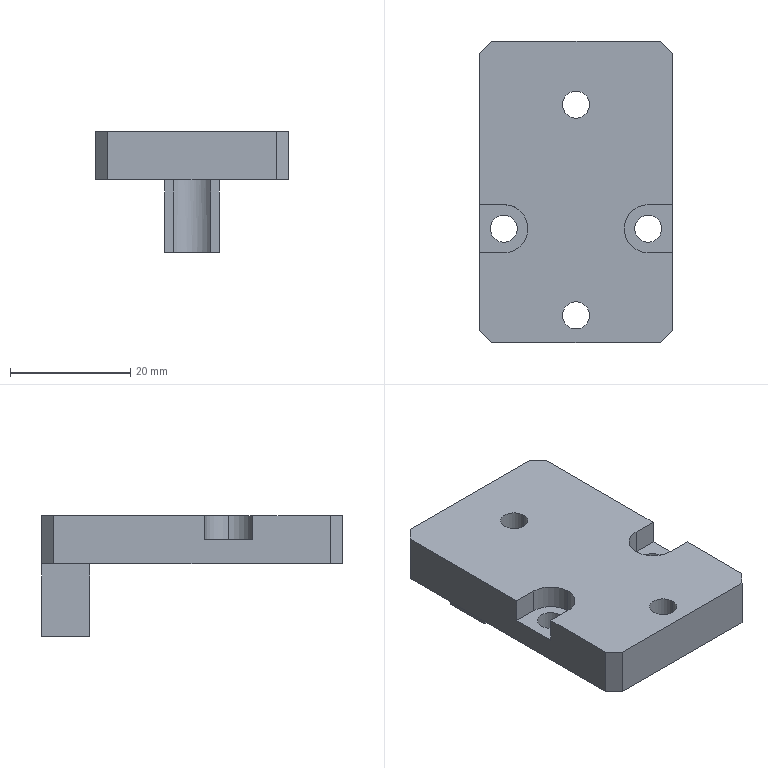Part | STEP file | 02-08 gripper limit block | 1 solid | 38 faces | box 32 x 50 x 20 mm | volume 12367 mm3 | plane 23 | cylinder 15 | commonest cylinder face diameters 4.5 x8 8 x7
STEP:
#1=CARTESIAN_POINT('',(4.,-20.5,16.6));
#2=VERTEX_POINT('',#1);
#3=CARTESIAN_POINT('',(-4.,-20.5,16.6));
#4=VERTEX_POINT('',#3);
#5=CARTESIAN_POINT('',(0.,-20.5,16.6));
#6=DIRECTION('',(0.,0.,-1.));
#7=DIRECTION('',(-1.,0.,0.));
#8=AXIS2_PLACEMENT_3D('',#5,#6,#7);
#9=CIRCLE('',#8,4.);
#10=EDGE_CURVE('',#2,#4,#9,.T.);
#11=ORIENTED_EDGE('',*,*,#10,.F.);
#12=CARTESIAN_POINT('',(4.,-20.5,12.));
#13=VERTEX_POINT('',#12);
#14=CARTESIAN_POINT('',(4.,-20.5,12.));
#15=DIRECTION('',(0.,0.,-1.));
#16=VECTOR('',#15,1000.);
#17=LINE('',#14,#16);
#18=EDGE_CURVE('',#2,#13,#17,.T.);
#19=ORIENTED_EDGE('',*,*,#18,.T.);
#20=CARTESIAN_POINT('',(-4.,-20.5,12.));
#21=VERTEX_POINT('',#20);
#22=CARTESIAN_POINT('',(0.,-20.5,12.));
#23=DIRECTION('',(0.,0.,-1.));
#24=DIRECTION('',(-1.,0.,0.));
#25=AXIS2_PLACEMENT_3D('',#22,#23,#24);
#26=CIRCLE('',#25,4.);
#27=EDGE_CURVE('',#13,#21,#26,.T.);
#28=ORIENTED_EDGE('',*,*,#27,.T.);
#29=CARTESIAN_POINT('',(-4.,-20.5,12.));
#30=DIRECTION('',(0.,0.,-1.));
#31=VECTOR('',#30,1000.);
#32=LINE('',#29,#31);
#33=EDGE_CURVE('',#4,#21,#32,.T.);
#34=ORIENTED_EDGE('',*,*,#33,.F.);
#35=EDGE_LOOP('',(#11,#19,#28,#34));
#36=FACE_OUTER_BOUND('',#35,.T.);
#37=CARTESIAN_POINT('',(0.,-20.5,12.));
#38=DIRECTION('',(0.,0.,-1.));
#39=DIRECTION('',(-1.,0.,0.));
#40=AXIS2_PLACEMENT_3D('',#37,#38,#39);
#41=CYLINDRICAL_SURFACE('',#40,4.);
#42=ADVANCED_FACE('',(#36),#41,.F.);
#43=CARTESIAN_POINT('',(2.25,-20.5,20.));
#44=VERTEX_POINT('',#43);
#45=CARTESIAN_POINT('',(-2.25,-20.5,20.));
#46=VERTEX_POINT('',#45);
#47=CARTESIAN_POINT('',(0.,-20.5,20.));
#48=DIRECTION('',(0.,0.,-1.));
#49=DIRECTION('',(-1.,0.,0.));
#50=AXIS2_PLACEMENT_3D('',#47,#48,#49);
#51=CIRCLE('',#50,2.25);
#52=EDGE_CURVE('',#44,#46,#51,.T.);
#53=ORIENTED_EDGE('',*,*,#52,.F.);
#54=CARTESIAN_POINT('',(2.25,-20.5,16.6));
#55=VERTEX_POINT('',#54);
#56=CARTESIAN_POINT('',(2.25,-20.5,12.));
#57=DIRECTION('',(0.,0.,-1.));
#58=VECTOR('',#57,1000.);
#59=LINE('',#56,#58);
#60=EDGE_CURVE('',#44,#55,#59,.T.);
#61=ORIENTED_EDGE('',*,*,#60,.T.);
#62=CARTESIAN_POINT('',(-2.25,-20.5,16.6));
#63=VERTEX_POINT('',#62);
#64=CARTESIAN_POINT('',(0.,-20.5,16.6));
#65=DIRECTION('',(0.,0.,-1.));
#66=DIRECTION('',(-1.,0.,0.));
#67=AXIS2_PLACEMENT_3D('',#64,#65,#66);
#68=CIRCLE('',#67,2.25);
#69=EDGE_CURVE('',#55,#63,#68,.T.);
#70=ORIENTED_EDGE('',*,*,#69,.T.);
#71=CARTESIAN_POINT('',(-2.25,-20.5,12.));
#72=DIRECTION('',(0.,0.,-1.));
#73=VECTOR('',#72,1000.);
#74=LINE('',#71,#73);
#75=EDGE_CURVE('',#46,#63,#74,.T.);
#76=ORIENTED_EDGE('',*,*,#75,.F.);
#77=EDGE_LOOP('',(#53,#61,#70,#76));
#78=FACE_OUTER_BOUND('',#77,.T.);
#79=CARTESIAN_POINT('',(0.,-20.5,12.));
#80=DIRECTION('',(0.,0.,-1.));
#81=DIRECTION('',(-1.,0.,0.));
#82=AXIS2_PLACEMENT_3D('',#79,#80,#81);
#83=CYLINDRICAL_SURFACE('',#82,2.25);
#84=ADVANCED_FACE('',(#78),#83,.F.);
#85=CARTESIAN_POINT('',(4.,14.5,16.6));
#86=VERTEX_POINT('',#85);
#87=CARTESIAN_POINT('',(-4.,14.5,16.6));
#88=VERTEX_POINT('',#87);
#89=CARTESIAN_POINT('',(0.,14.5,16.6));
#90=DIRECTION('',(0.,0.,-1.));
#91=DIRECTION('',(-1.,0.,0.));
#92=AXIS2_PLACEMENT_3D('',#89,#90,#91);
#93=CIRCLE('',#92,4.);
#94=EDGE_CURVE('',#86,#88,#93,.T.);
#95=ORIENTED_EDGE('',*,*,#94,.F.);
#96=CARTESIAN_POINT('',(4.,14.5,12.));
#97=VERTEX_POINT('',#96);
#98=CARTESIAN_POINT('',(4.,14.5,12.));
#99=DIRECTION('',(0.,0.,-1.));
#100=VECTOR('',#99,1000.);
#101=LINE('',#98,#100);
#102=EDGE_CURVE('',#86,#97,#101,.T.);
#103=ORIENTED_EDGE('',*,*,#102,.T.);
#104=CARTESIAN_POINT('',(-4.,14.5,12.));
#105=VERTEX_POINT('',#104);
#106=CARTESIAN_POINT('',(0.,14.5,12.));
#107=DIRECTION('',(0.,0.,-1.));
#108=DIRECTION('',(-1.,0.,0.));
#109=AXIS2_PLACEMENT_3D('',#106,#107,#108);
#110=CIRCLE('',#109,4.);
#111=EDGE_CURVE('',#97,#105,#110,.T.);
#112=ORIENTED_EDGE('',*,*,#111,.T.);
#113=CARTESIAN_POINT('',(-4.,14.5,12.));
#114=DIRECTION('',(0.,0.,-1.));
#115=VECTOR('',#114,1000.);
#116=LINE('',#113,#115);
#117=EDGE_CURVE('',#88,#105,#116,.T.);
#118=ORIENTED_EDGE('',*,*,#117,.F.);
#119=EDGE_LOOP('',(#95,#103,#112,#118));
#120=FACE_OUTER_BOUND('',#119,.T.);
#121=CARTESIAN_POINT('',(0.,14.5,12.));
#122=DIRECTION('',(0.,0.,-1.));
#123=DIRECTION('',(-1.,0.,0.));
#124=AXIS2_PLACEMENT_3D('',#121,#122,#123);
#125=CYLINDRICAL_SURFACE('',#124,4.);
#126=ADVANCED_FACE('',(#120),#125,.F.);
#127=CARTESIAN_POINT('',(2.25,14.5,20.));
#128=VERTEX_POINT('',#127);
#129=CARTESIAN_POINT('',(-2.25,14.5,20.));
#130=VERTEX_POINT('',#129);
#131=CARTESIAN_POINT('',(0.,14.5,20.));
#132=DIRECTION('',(0.,0.,-1.));
#133=DIRECTION('',(-1.,0.,0.));
#134=AXIS2_PLACEMENT_3D('',#131,#132,#133);
#135=CIRCLE('',#134,2.25);
#136=EDGE_CURVE('',#128,#130,#135,.T.);
#137=ORIENTED_EDGE('',*,*,#136,.F.);
#138=CARTESIAN_POINT('',(2.25,14.5,16.6));
#139=VERTEX_POINT('',#138);
#140=CARTESIAN_POINT('',(2.25,14.5,12.));
#141=DIRECTION('',(0.,0.,-1.));
#142=VECTOR('',#141,1000.);
#143=LINE('',#140,#142);
#144=EDGE_CURVE('',#128,#139,#143,.T.);
#145=ORIENTED_EDGE('',*,*,#144,.T.);
#146=CARTESIAN_POINT('',(-2.25,14.5,16.6));
#147=VERTEX_POINT('',#146);
#148=CARTESIAN_POINT('',(0.,14.5,16.6));
#149=DIRECTION('',(0.,0.,-1.));
#150=DIRECTION('',(-1.,0.,0.));
#151=AXIS2_PLACEMENT_3D('',#148,#149,#150);
#152=CIRCLE('',#151,2.25);
#153=EDGE_CURVE('',#139,#147,#152,.T.);
#154=ORIENTED_EDGE('',*,*,#153,.T.);
#155=CARTESIAN_POINT('',(-2.25,14.5,12.));
#156=DIRECTION('',(0.,0.,-1.));
#157=VECTOR('',#156,1000.);
#158=LINE('',#155,#157);
#159=EDGE_CURVE('',#130,#147,#158,.T.);
#160=ORIENTED_EDGE('',*,*,#159,.F.);
#161=EDGE_LOOP('',(#137,#145,#154,#160));
#162=FACE_OUTER_BOUND('',#161,.T.);
#163=CARTESIAN_POINT('',(0.,14.5,12.));
#164=DIRECTION('',(0.,0.,-1.));
#165=DIRECTION('',(-1.,0.,0.));
#166=AXIS2_PLACEMENT_3D('',#163,#164,#165);
#167=CYLINDRICAL_SURFACE('',#166,2.25);
#168=ADVANCED_FACE('',(#162),#167,.F.);
#169=CARTESIAN_POINT('',(-8.,-6.1,16.));
#170=VERTEX_POINT('',#169);
#171=CARTESIAN_POINT('',(-12.,-2.1,16.));
#172=VERTEX_POINT('',#171);
#173=CARTESIAN_POINT('',(-12.,-6.1,16.));
#174=DIRECTION('',(0.,0.,1.));
#175=DIRECTION('',(1.,0.,0.));
#176=AXIS2_PLACEMENT_3D('',#173,#174,#175);
#177=CIRCLE('',#176,4.);
#178=EDGE_CURVE('',#170,#172,#177,.T.);
#179=ORIENTED_EDGE('',*,*,#178,.F.);
#180=CARTESIAN_POINT('',(-8.,-6.1,20.));
#181=VERTEX_POINT('',#180);
#182=CARTESIAN_POINT('',(-8.,-6.1,16.));
#183=DIRECTION('',(0.,0.,1.));
#184=VECTOR('',#183,1000.);
#185=LINE('',#182,#184);
#186=EDGE_CURVE('',#170,#181,#185,.T.);
#187=ORIENTED_EDGE('',*,*,#186,.T.);
#188=CARTESIAN_POINT('',(-12.,-2.1,20.));
#189=VERTEX_POINT('',#188);
#190=CARTESIAN_POINT('',(-12.,-6.1,20.));
#191=DIRECTION('',(0.,0.,1.));
#192=DIRECTION('',(1.,0.,0.));
#193=AXIS2_PLACEMENT_3D('',#190,#191,#192);
#194=CIRCLE('',#193,4.);
#195=EDGE_CURVE('',#181,#189,#194,.T.);
#196=ORIENTED_EDGE('',*,*,#195,.T.);
#197=CARTESIAN_POINT('',(-12.,-2.1,16.));
#198=DIRECTION('',(0.,0.,1.));
#199=VECTOR('',#198,1000.);
#200=LINE('',#197,#199);
#201=EDGE_CURVE('',#172,#189,#200,.T.);
#202=ORIENTED_EDGE('',*,*,#201,.F.);
#203=EDGE_LOOP('',(#179,#187,#196,#202));
#204=FACE_OUTER_BOUND('',#203,.T.);
#205=CARTESIAN_POINT('',(-12.,-6.1,16.));
#206=DIRECTION('',(0.,0.,1.));
#207=DIRECTION('',(1.,0.,0.));
#208=AXIS2_PLACEMENT_3D('',#205,#206,#207);
#209=CYLINDRICAL_SURFACE('',#208,4.);
#210=ADVANCED_FACE('',(#204),#209,.F.);
#211=CARTESIAN_POINT('',(9.75,-6.1,12.));
#212=VERTEX_POINT('',#211);
#213=CARTESIAN_POINT('',(14.25,-6.1,12.));
#214=VERTEX_POINT('',#213);
#215=CARTESIAN_POINT('',(12.,-6.1,12.));
#216=DIRECTION('',(0.,0.,1.));
#217=DIRECTION('',(1.,0.,0.));
#218=AXIS2_PLACEMENT_3D('',#215,#216,#217);
#219=CIRCLE('',#218,2.25);
#220=EDGE_CURVE('',#212,#214,#219,.T.);
#221=ORIENTED_EDGE('',*,*,#220,.F.);
#222=CARTESIAN_POINT('',(9.75,-6.1,16.));
#223=VERTEX_POINT('',#222);
#224=CARTESIAN_POINT('',(9.75,-6.1,-10.));
#225=DIRECTION('',(0.,0.,1.));
#226=VECTOR('',#225,1000.);
#227=LINE('',#224,#226);
#228=EDGE_CURVE('',#212,#223,#227,.T.);
#229=ORIENTED_EDGE('',*,*,#228,.T.);
#230=CARTESIAN_POINT('',(14.25,-6.1,16.));
#231=VERTEX_POINT('',#230);
#232=CARTESIAN_POINT('',(12.,-6.1,16.));
#233=DIRECTION('',(0.,0.,-1.));
#234=DIRECTION('',(1.,0.,0.));
#235=AXIS2_PLACEMENT_3D('',#232,#233,#234);
#236=CIRCLE('',#235,2.25);
#237=EDGE_CURVE('',#231,#223,#236,.T.);
#238=ORIENTED_EDGE('',*,*,#237,.F.);
#239=CARTESIAN_POINT('',(14.25,-6.1,-10.));
#240=DIRECTION('',(0.,0.,1.));
#241=VECTOR('',#240,1000.);
#242=LINE('',#239,#241);
#243=EDGE_CURVE('',#214,#231,#242,.T.);
#244=ORIENTED_EDGE('',*,*,#243,.F.);
#245=EDGE_LOOP('',(#221,#229,#238,#244));
#246=FACE_OUTER_BOUND('',#245,.T.);
#247=CARTESIAN_POINT('',(12.,-6.1,-10.));
#248=DIRECTION('',(0.,0.,1.));
#249=DIRECTION('',(1.,0.,0.));
#250=AXIS2_PLACEMENT_3D('',#247,#248,#249);
#251=CYLINDRICAL_SURFACE('',#250,2.25);
#252=ADVANCED_FACE('',(#246),#251,.F.);
#253=CARTESIAN_POINT('',(-14.25,-6.1,12.));
#254=VERTEX_POINT('',#253);
#255=CARTESIAN_POINT('',(-9.75,-6.1,12.));
#256=VERTEX_POINT('',#255);
#257=CARTESIAN_POINT('',(-12.,-6.1,12.));
#258=DIRECTION('',(0.,0.,1.));
#259=DIRECTION('',(1.,0.,0.));
#260=AXIS2_PLACEMENT_3D('',#257,#258,#259);
#261=CIRCLE('',#260,2.25);
#262=EDGE_CURVE('',#254,#256,#261,.T.);
#263=ORIENTED_EDGE('',*,*,#262,.F.);
#264=CARTESIAN_POINT('',(-14.25,-6.1,16.));
#265=VERTEX_POINT('',#264);
#266=CARTESIAN_POINT('',(-14.25,-6.1,-10.));
#267=DIRECTION('',(0.,0.,1.));
#268=VECTOR('',#267,1000.);
#269=LINE('',#266,#268);
#270=EDGE_CURVE('',#254,#265,#269,.T.);
#271=ORIENTED_EDGE('',*,*,#270,.T.);
#272=CARTESIAN_POINT('',(-9.75,-6.1,16.));
#273=VERTEX_POINT('',#272);
#274=CARTESIAN_POINT('',(-12.,-6.1,16.));
#275=DIRECTION('',(0.,0.,-1.));
#276=DIRECTION('',(1.,0.,0.));
#277=AXIS2_PLACEMENT_3D('',#274,#275,#276);
#278=CIRCLE('',#277,2.25);
#279=EDGE_CURVE('',#273,#265,#278,.T.);
#280=ORIENTED_EDGE('',*,*,#279,.F.);
#281=CARTESIAN_POINT('',(-9.75,-6.1,-10.));
#282=DIRECTION('',(0.,0.,1.));
#283=VECTOR('',#282,1000.);
#284=LINE('',#281,#283);
#285=EDGE_CURVE('',#256,#273,#284,.T.);
#286=ORIENTED_EDGE('',*,*,#285,.F.);
#287=EDGE_LOOP('',(#263,#271,#280,#286));
#288=FACE_OUTER_BOUND('',#287,.T.);
#289=CARTESIAN_POINT('',(-12.,-6.1,-10.));
#290=DIRECTION('',(0.,0.,1.));
#291=DIRECTION('',(1.,0.,0.));
#292=AXIS2_PLACEMENT_3D('',#289,#290,#291);
#293=CYLINDRICAL_SURFACE('',#292,2.25);
#294=ADVANCED_FACE('',(#288),#293,.F.);
#295=CARTESIAN_POINT('',(-3.122,17.,0.));
#296=VERTEX_POINT('',#295);
#297=CARTESIAN_POINT('',(3.122,17.,0.));
#298=VERTEX_POINT('',#297);
#299=CARTESIAN_POINT('',(0.,14.5,0.));
#300=DIRECTION('',(0.,0.,-1.));
#301=DIRECTION('',(1.,0.,0.));
#302=AXIS2_PLACEMENT_3D('',#299,#300,#301);
#303=CIRCLE('',#302,4.);
#304=EDGE_CURVE('',#296,#298,#303,.T.);
#305=ORIENTED_EDGE('',*,*,#304,.F.);
#306=CARTESIAN_POINT('',(-4.5,17.,0.));
#307=VERTEX_POINT('',#306);
#308=CARTESIAN_POINT('',(34.,17.,0.));
#309=DIRECTION('',(-1.,0.,0.));
#310=VECTOR('',#309,1000.);
#311=LINE('',#308,#310);
#312=EDGE_CURVE('',#296,#307,#311,.T.);
#313=ORIENTED_EDGE('',*,*,#312,.T.);
#314=CARTESIAN_POINT('',(-4.5,25.,0.));
#315=VERTEX_POINT('',#314);
#316=CARTESIAN_POINT('',(-4.5,25.,0.));
#317=DIRECTION('',(0.,1.,0.));
#318=VECTOR('',#317,1000.);
#319=LINE('',#316,#318);
#320=EDGE_CURVE('',#307,#315,#319,.T.);
#321=ORIENTED_EDGE('',*,*,#320,.T.);
#322=CARTESIAN_POINT('',(4.5,25.,0.));
#323=VERTEX_POINT('',#322);
#324=CARTESIAN_POINT('',(-16.,25.,0.));
#325=DIRECTION('',(-1.,0.,0.));
#326=VECTOR('',#325,1000.);
#327=LINE('',#324,#326);
#328=EDGE_CURVE('',#323,#315,#327,.T.);
#329=ORIENTED_EDGE('',*,*,#328,.F.);
#330=CARTESIAN_POINT('',(4.5,17.,0.));
#331=VERTEX_POINT('',#330);
#332=CARTESIAN_POINT('',(4.5,25.,0.));
#333=DIRECTION('',(0.,-1.,0.));
#334=VECTOR('',#333,1000.);
#335=LINE('',#332,#334);
#336=EDGE_CURVE('',#323,#331,#335,.T.);
#337=ORIENTED_EDGE('',*,*,#336,.T.);
#338=CARTESIAN_POINT('',(34.,17.,0.));
#339=DIRECTION('',(-1.,0.,0.));
#340=VECTOR('',#339,1000.);
#341=LINE('',#338,#340);
#342=EDGE_CURVE('',#331,#298,#341,.T.);
#343=ORIENTED_EDGE('',*,*,#342,.T.);
#344=EDGE_LOOP('',(#305,#313,#321,#329,#337,#343));
#345=FACE_OUTER_BOUND('',#344,.T.);
#346=CARTESIAN_POINT('',(16.,-25.,0.));
#347=DIRECTION('',(0.,0.,1.));
#348=DIRECTION('',(1.,0.,0.));
#349=AXIS2_PLACEMENT_3D('',#346,#347,#348);
#350=PLANE('',#349);
#351=ADVANCED_FACE('',(#345),#350,.F.);
#352=CARTESIAN_POINT('',(-3.122,17.,12.));
#353=VERTEX_POINT('',#352);
#354=CARTESIAN_POINT('',(-3.122,17.,-2.4));
#355=DIRECTION('',(0.,0.,-1.));
#356=VECTOR('',#355,1000.);
#357=LINE('',#354,#356);
#358=EDGE_CURVE('',#353,#296,#357,.T.);
#359=ORIENTED_EDGE('',*,*,#358,.F.);
#360=CARTESIAN_POINT('',(-4.5,17.,12.));
#361=VERTEX_POINT('',#360);
#362=CARTESIAN_POINT('',(34.,17.,12.));
#363=DIRECTION('',(-1.,0.,0.));
#364=VECTOR('',#363,1000.);
#365=LINE('',#362,#364);
#366=EDGE_CURVE('',#353,#361,#365,.T.);
#367=ORIENTED_EDGE('',*,*,#366,.T.);
#368=CARTESIAN_POINT('',(-4.5,17.,0.));
#369=DIRECTION('',(0.,0.,1.));
#370=VECTOR('',#369,1000.);
#371=LINE('',#368,#370);
#372=EDGE_CURVE('',#307,#361,#371,.T.);
#373=ORIENTED_EDGE('',*,*,#372,.F.);
#374=ORIENTED_EDGE('',*,*,#312,.F.);
#375=EDGE_LOOP('',(#359,#367,#373,#374));
#376=FACE_OUTER_BOUND('',#375,.T.);
#377=CARTESIAN_POINT('',(34.,17.,0.));
#378=DIRECTION('',(0.,1.,0.));
#379=DIRECTION('',(-1.,0.,0.));
#380=AXIS2_PLACEMENT_3D('',#377,#378,#379);
#381=PLANE('',#380);
#382=ADVANCED_FACE('',(#376),#381,.F.);
#383=CARTESIAN_POINT('',(3.122,17.,12.));
#384=VERTEX_POINT('',#383);
#385=CARTESIAN_POINT('',(3.122,17.,-2.4));
#386=DIRECTION('',(0.,0.,1.));
#387=VECTOR('',#386,1000.);
#388=LINE('',#385,#387);
#389=EDGE_CURVE('',#298,#384,#388,.T.);
#390=ORIENTED_EDGE('',*,*,#389,.F.);
#391=ORIENTED_EDGE('',*,*,#342,.F.);
#392=CARTESIAN_POINT('',(4.5,17.,12.));
#393=VERTEX_POINT('',#392);
#394=CARTESIAN_POINT('',(4.5,17.,0.));
#395=DIRECTION('',(0.,0.,-1.));
#396=VECTOR('',#395,1000.);
#397=LINE('',#394,#396);
#398=EDGE_CURVE('',#393,#331,#397,.T.);
#399=ORIENTED_EDGE('',*,*,#398,.F.);
#400=CARTESIAN_POINT('',(34.,17.,12.));
#401=DIRECTION('',(-1.,0.,0.));
#402=VECTOR('',#401,1000.);
#403=LINE('',#400,#402);
#404=EDGE_CURVE('',#393,#384,#403,.T.);
#405=ORIENTED_EDGE('',*,*,#404,.T.);
#406=EDGE_LOOP('',(#390,#391,#399,#405));
#407=FACE_OUTER_BOUND('',#406,.T.);
#408=CARTESIAN_POINT('',(34.,17.,0.));
#409=DIRECTION('',(0.,1.,0.));
#410=DIRECTION('',(-1.,0.,0.));
#411=AXIS2_PLACEMENT_3D('',#408,#409,#410);
#412=PLANE('',#411);
#413=ADVANCED_FACE('',(#407),#412,.F.);
#414=CARTESIAN_POINT('',(0.,-20.5,12.));
#415=DIRECTION('',(0.,0.,-1.));
#416=DIRECTION('',(-1.,0.,0.));
#417=AXIS2_PLACEMENT_3D('',#414,#415,#416);
#418=CIRCLE('',#417,4.);
#419=EDGE_CURVE('',#21,#13,#418,.T.);
#420=ORIENTED_EDGE('',*,*,#419,.F.);
#421=ORIENTED_EDGE('',*,*,#27,.F.);
#422=EDGE_LOOP('',(#420,#421));
#423=FACE_BOUND('',#422,.T.);
#424=CARTESIAN_POINT('',(12.,-6.1,12.));
#425=DIRECTION('',(0.,0.,1.));
#426=DIRECTION('',(1.,0.,0.));
#427=AXIS2_PLACEMENT_3D('',#424,#425,#426);
#428=CIRCLE('',#427,2.25);
#429=EDGE_CURVE('',#214,#212,#428,.T.);
#430=ORIENTED_EDGE('',*,*,#429,.T.);
#431=ORIENTED_EDGE('',*,*,#220,.T.);
#432=EDGE_LOOP('',(#430,#431));
#433=FACE_BOUND('',#432,.T.);
#434=CARTESIAN_POINT('',(-12.,-6.1,12.));
#435=DIRECTION('',(0.,0.,1.));
#436=DIRECTION('',(1.,0.,0.));
#437=AXIS2_PLACEMENT_3D('',#434,#435,#436);
#438=CIRCLE('',#437,2.25);
#439=EDGE_CURVE('',#256,#254,#438,.T.);
#440=ORIENTED_EDGE('',*,*,#439,.T.);
#441=ORIENTED_EDGE('',*,*,#262,.T.);
#442=EDGE_LOOP('',(#440,#441));
#443=FACE_BOUND('',#442,.T.);
#444=CARTESIAN_POINT('',(0.,14.5,12.));
#445=DIRECTION('',(0.,0.,-1.));
#446=DIRECTION('',(-1.,0.,0.));
#447=AXIS2_PLACEMENT_3D('',#444,#445,#446);
#448=CIRCLE('',#447,4.);
#449=EDGE_CURVE('',#384,#97,#448,.T.);
#450=ORIENTED_EDGE('',*,*,#449,.F.);
#451=ORIENTED_EDGE('',*,*,#404,.F.);
#452=CARTESIAN_POINT('',(4.5,25.,12.));
#453=VERTEX_POINT('',#452);
#454=CARTESIAN_POINT('',(4.5,25.,12.));
#455=DIRECTION('',(0.,1.,0.));
#456=VECTOR('',#455,1000.);
#457=LINE('',#454,#456);
#458=EDGE_CURVE('',#393,#453,#457,.T.);
#459=ORIENTED_EDGE('',*,*,#458,.T.);
#460=CARTESIAN_POINT('',(14.,25.,12.));
#461=VERTEX_POINT('',#460);
#462=CARTESIAN_POINT('',(16.,25.,12.));
#463=DIRECTION('',(1.,0.,0.));
#464=VECTOR('',#463,1000.);
#465=LINE('',#462,#464);
#466=EDGE_CURVE('',#453,#461,#465,.T.);
#467=ORIENTED_EDGE('',*,*,#466,.T.);
#468=CARTESIAN_POINT('',(16.,23.,12.));
#469=VERTEX_POINT('',#468);
#470=CARTESIAN_POINT('',(14.,25.,12.));
#471=DIRECTION('',(0.7071,-0.7071,0.));
#472=VECTOR('',#471,1000.);
#473=LINE('',#470,#472);
#474=EDGE_CURVE('',#461,#469,#473,.T.);
#475=ORIENTED_EDGE('',*,*,#474,.T.);
#476=CARTESIAN_POINT('',(16.,-23.,12.));
#477=VERTEX_POINT('',#476);
#478=CARTESIAN_POINT('',(16.,25.,12.));
#479=DIRECTION('',(0.,1.,0.));
#480=VECTOR('',#479,1000.);
#481=LINE('',#478,#480);
#482=EDGE_CURVE('',#477,#469,#481,.T.);
#483=ORIENTED_EDGE('',*,*,#482,.F.);
#484=CARTESIAN_POINT('',(14.,-25.,12.));
#485=VERTEX_POINT('',#484);
#486=CARTESIAN_POINT('',(16.,-23.,12.));
#487=DIRECTION('',(-0.7071,-0.7071,0.));
#488=VECTOR('',#487,1000.);
#489=LINE('',#486,#488);
#490=EDGE_CURVE('',#477,#485,#489,.T.);
#491=ORIENTED_EDGE('',*,*,#490,.T.);
#492=CARTESIAN_POINT('',(-14.,-25.,12.));
#493=VERTEX_POINT('',#492);
#494=CARTESIAN_POINT('',(34.,-25.,12.));
#495=DIRECTION('',(-1.,0.,0.));
#496=VECTOR('',#495,1000.);
#497=LINE('',#494,#496);
#498=EDGE_CURVE('',#485,#493,#497,.T.);
#499=ORIENTED_EDGE('',*,*,#498,.T.);
#500=CARTESIAN_POINT('',(-16.,-23.,12.));
#501=VERTEX_POINT('',#500);
#502=CARTESIAN_POINT('',(-14.,-25.,12.));
#503=DIRECTION('',(-0.7071,0.7071,0.));
#504=VECTOR('',#503,1000.);
#505=LINE('',#502,#504);
#506=EDGE_CURVE('',#493,#501,#505,.T.);
#507=ORIENTED_EDGE('',*,*,#506,.T.);
#508=CARTESIAN_POINT('',(-16.,23.,12.));
#509=VERTEX_POINT('',#508);
#510=CARTESIAN_POINT('',(-16.,-25.,12.));
#511=DIRECTION('',(0.,1.,0.));
#512=VECTOR('',#511,1000.);
#513=LINE('',#510,#512);
#514=EDGE_CURVE('',#501,#509,#513,.T.);
#515=ORIENTED_EDGE('',*,*,#514,.T.);
#516=CARTESIAN_POINT('',(-14.,25.,12.));
#517=VERTEX_POINT('',#516);
#518=CARTESIAN_POINT('',(-16.,23.,12.));
#519=DIRECTION('',(0.7071,0.7071,0.));
#520=VECTOR('',#519,1000.);
#521=LINE('',#518,#520);
#522=EDGE_CURVE('',#509,#517,#521,.T.);
#523=ORIENTED_EDGE('',*,*,#522,.T.);
#524=CARTESIAN_POINT('',(-4.5,25.,12.));
#525=VERTEX_POINT('',#524);
#526=CARTESIAN_POINT('',(16.,25.,12.));
#527=DIRECTION('',(1.,0.,0.));
#528=VECTOR('',#527,1000.);
#529=LINE('',#526,#528);
#530=EDGE_CURVE('',#517,#525,#529,.T.);
#531=ORIENTED_EDGE('',*,*,#530,.T.);
#532=CARTESIAN_POINT('',(-4.5,25.,12.));
#533=DIRECTION('',(0.,-1.,0.));
#534=VECTOR('',#533,1000.);
#535=LINE('',#532,#534);
#536=EDGE_CURVE('',#525,#361,#535,.T.);
#537=ORIENTED_EDGE('',*,*,#536,.T.);
#538=ORIENTED_EDGE('',*,*,#366,.F.);
#539=CARTESIAN_POINT('',(0.,14.5,12.));
#540=DIRECTION('',(0.,0.,-1.));
#541=DIRECTION('',(-1.,0.,0.));
#542=AXIS2_PLACEMENT_3D('',#539,#540,#541);
#543=CIRCLE('',#542,4.);
#544=EDGE_CURVE('',#105,#353,#543,.T.);
#545=ORIENTED_EDGE('',*,*,#544,.F.);
#546=ORIENTED_EDGE('',*,*,#111,.F.);
#547=EDGE_LOOP('',(#450,#451,#459,#467,#475,#483,#491,#499,#507,#515,#523,#531,#537,#538,#545,#546));
#548=FACE_OUTER_BOUND('',#547,.T.);
#549=CARTESIAN_POINT('',(34.,-25.,12.));
#550=DIRECTION('',(0.,0.,1.));
#551=DIRECTION('',(1.,0.,0.));
#552=AXIS2_PLACEMENT_3D('',#549,#550,#551);
#553=PLANE('',#552);
#554=ADVANCED_FACE('',(#423,#433,#443,#548),#553,.F.);
#555=ORIENTED_EDGE('',*,*,#458,.F.);
#556=ORIENTED_EDGE('',*,*,#398,.T.);
#557=ORIENTED_EDGE('',*,*,#336,.F.);
#558=CARTESIAN_POINT('',(4.5,25.,0.));
#559=DIRECTION('',(0.,0.,1.));
#560=VECTOR('',#559,1000.);
#561=LINE('',#558,#560);
#562=EDGE_CURVE('',#323,#453,#561,.T.);
#563=ORIENTED_EDGE('',*,*,#562,.T.);
#564=EDGE_LOOP('',(#555,#556,#557,#563));
#565=FACE_OUTER_BOUND('',#564,.T.);
#566=CARTESIAN_POINT('',(4.5,25.,0.));
#567=DIRECTION('',(-1.,0.,0.));
#568=DIRECTION('',(0.,-1.,0.));
#569=AXIS2_PLACEMENT_3D('',#566,#567,#568);
#570=PLANE('',#569);
#571=ADVANCED_FACE('',(#565),#570,.F.);
#572=ORIENTED_EDGE('',*,*,#536,.F.);
#573=CARTESIAN_POINT('',(-4.5,25.,0.));
#574=DIRECTION('',(0.,0.,1.));
#575=VECTOR('',#574,1000.);
#576=LINE('',#573,#575);
#577=EDGE_CURVE('',#315,#525,#576,.T.);
#578=ORIENTED_EDGE('',*,*,#577,.F.);
#579=ORIENTED_EDGE('',*,*,#320,.F.);
#580=ORIENTED_EDGE('',*,*,#372,.T.);
#581=EDGE_LOOP('',(#572,#578,#579,#580));
#582=FACE_OUTER_BOUND('',#581,.T.);
#583=CARTESIAN_POINT('',(-4.5,25.,0.));
#584=DIRECTION('',(1.,0.,0.));
#585=DIRECTION('',(0.,1.,0.));
#586=AXIS2_PLACEMENT_3D('',#583,#584,#585);
#587=PLANE('',#586);
#588=ADVANCED_FACE('',(#582),#587,.F.);
#589=ORIENTED_EDGE('',*,*,#270,.F.);
#590=ORIENTED_EDGE('',*,*,#439,.F.);
#591=ORIENTED_EDGE('',*,*,#285,.T.);
#592=CARTESIAN_POINT('',(-12.,-6.1,16.));
#593=DIRECTION('',(0.,0.,-1.));
#594=DIRECTION('',(1.,0.,0.));
#595=AXIS2_PLACEMENT_3D('',#592,#593,#594);
#596=CIRCLE('',#595,2.25);
#597=EDGE_CURVE('',#265,#273,#596,.T.);
#598=ORIENTED_EDGE('',*,*,#597,.F.);
#599=EDGE_LOOP('',(#589,#590,#591,#598));
#600=FACE_OUTER_BOUND('',#599,.T.);
#601=CARTESIAN_POINT('',(-12.,-6.1,-10.));
#602=DIRECTION('',(0.,0.,1.));
#603=DIRECTION('',(1.,0.,0.));
#604=AXIS2_PLACEMENT_3D('',#601,#602,#603);
#605=CYLINDRICAL_SURFACE('',#604,2.25);
#606=ADVANCED_FACE('',(#600),#605,.F.);
#607=ORIENTED_EDGE('',*,*,#228,.F.);
#608=ORIENTED_EDGE('',*,*,#429,.F.);
#609=ORIENTED_EDGE('',*,*,#243,.T.);
#610=CARTESIAN_POINT('',(12.,-6.1,16.));
#611=DIRECTION('',(0.,0.,-1.));
#612=DIRECTION('',(1.,0.,0.));
#613=AXIS2_PLACEMENT_3D('',#610,#611,#612);
#614=CIRCLE('',#613,2.25);
#615=EDGE_CURVE('',#223,#231,#614,.T.);
#616=ORIENTED_EDGE('',*,*,#615,.F.);
#617=EDGE_LOOP('',(#607,#608,#609,#616));
#618=FACE_OUTER_BOUND('',#617,.T.);
#619=CARTESIAN_POINT('',(12.,-6.1,-10.));
#620=DIRECTION('',(0.,0.,1.));
#621=DIRECTION('',(1.,0.,0.));
#622=AXIS2_PLACEMENT_3D('',#619,#620,#621);
#623=CYLINDRICAL_SURFACE('',#622,2.25);
#624=ADVANCED_FACE('',(#618),#623,.F.);
#625=CARTESIAN_POINT('',(16.,-23.,20.));
#626=VERTEX_POINT('',#625);
#627=CARTESIAN_POINT('',(16.,-10.1,20.));
#628=VERTEX_POINT('',#627);
#629=CARTESIAN_POINT('',(16.,25.,20.));
#630=DIRECTION('',(0.,1.,0.));
#631=VECTOR('',#630,1000.);
#632=LINE('',#629,#631);
#633=EDGE_CURVE('',#626,#628,#632,.T.);
#634=ORIENTED_EDGE('',*,*,#633,.F.);
#635=CARTESIAN_POINT('',(16.,-23.,20.));
#636=DIRECTION('',(0.,0.,-1.));
#637=VECTOR('',#636,1000.);
#638=LINE('',#635,#637);
#639=EDGE_CURVE('',#626,#477,#638,.T.);
#640=ORIENTED_EDGE('',*,*,#639,.T.);
#641=ORIENTED_EDGE('',*,*,#482,.T.);
#642=CARTESIAN_POINT('',(16.,23.,20.));
#643=VERTEX_POINT('',#642);
#644=CARTESIAN_POINT('',(16.,23.,20.));
#645=DIRECTION('',(0.,0.,1.));
#646=VECTOR('',#645,1000.);
#647=LINE('',#644,#646);
#648=EDGE_CURVE('',#469,#643,#647,.T.);
#649=ORIENTED_EDGE('',*,*,#648,.T.);
#650=CARTESIAN_POINT('',(16.,-2.1,20.));
#651=VERTEX_POINT('',#650);
#652=CARTESIAN_POINT('',(16.,25.,20.));
#653=DIRECTION('',(0.,1.,0.));
#654=VECTOR('',#653,1000.);
#655=LINE('',#652,#654);
#656=EDGE_CURVE('',#651,#643,#655,.T.);
#657=ORIENTED_EDGE('',*,*,#656,.F.);
#658=CARTESIAN_POINT('',(16.,-2.1,16.));
#659=VERTEX_POINT('',#658);
#660=CARTESIAN_POINT('',(16.,-2.1,20.));
#661=DIRECTION('',(0.,0.,-1.));
#662=VECTOR('',#661,1000.);
#663=LINE('',#660,#662);
#664=EDGE_CURVE('',#651,#659,#663,.T.);
#665=ORIENTED_EDGE('',*,*,#664,.T.);
#666=CARTESIAN_POINT('',(16.,-10.1,16.));
#667=VERTEX_POINT('',#666);
#668=CARTESIAN_POINT('',(16.,25.,16.));
#669=DIRECTION('',(0.,1.,0.));
#670=VECTOR('',#669,1000.);
#671=LINE('',#668,#670);
#672=EDGE_CURVE('',#667,#659,#671,.T.);
#673=ORIENTED_EDGE('',*,*,#672,.F.);
#674=CARTESIAN_POINT('',(16.,-10.1,20.));
#675=DIRECTION('',(0.,0.,1.));
#676=VECTOR('',#675,1000.);
#677=LINE('',#674,#676);
#678=EDGE_CURVE('',#667,#628,#677,.T.);
#679=ORIENTED_EDGE('',*,*,#678,.T.);
#680=EDGE_LOOP('',(#634,#640,#641,#649,#657,#665,#673,#679));
#681=FACE_OUTER_BOUND('',#680,.T.);
#682=CARTESIAN_POINT('',(16.,25.,20.));
#683=DIRECTION('',(-1.,0.,0.));
#684=DIRECTION('',(0.,-1.,0.));
#685=AXIS2_PLACEMENT_3D('',#682,#683,#684);
#686=PLANE('',#685);
#687=ADVANCED_FACE('',(#681),#686,.F.);
#688=CARTESIAN_POINT('',(14.,25.,20.));
#689=VERTEX_POINT('',#688);
#690=CARTESIAN_POINT('',(-14.,25.,20.));
#691=VERTEX_POINT('',#690);
#692=CARTESIAN_POINT('',(-16.,25.,20.));
#693=DIRECTION('',(-1.,0.,0.));
#694=VECTOR('',#693,1000.);
#695=LINE('',#692,#694);
#696=EDGE_CURVE('',#689,#691,#695,.T.);
#697=ORIENTED_EDGE('',*,*,#696,.F.);
#698=CARTESIAN_POINT('',(14.,25.,20.));
#699=DIRECTION('',(0.,0.,-1.));
#700=VECTOR('',#699,1000.);
#701=LINE('',#698,#700);
#702=EDGE_CURVE('',#689,#461,#701,.T.);
#703=ORIENTED_EDGE('',*,*,#702,.T.);
#704=ORIENTED_EDGE('',*,*,#466,.F.);
#705=ORIENTED_EDGE('',*,*,#562,.F.);
#706=ORIENTED_EDGE('',*,*,#328,.T.);
#707=ORIENTED_EDGE('',*,*,#577,.T.);
#708=ORIENTED_EDGE('',*,*,#530,.F.);
#709=CARTESIAN_POINT('',(-14.,25.,20.));
#710=DIRECTION('',(0.,0.,1.));
#711=VECTOR('',#710,1000.);
#712=LINE('',#709,#711);
#713=EDGE_CURVE('',#517,#691,#712,.T.);
#714=ORIENTED_EDGE('',*,*,#713,.T.);
#715=EDGE_LOOP('',(#697,#703,#704,#705,#706,#707,#708,#714));
#716=FACE_OUTER_BOUND('',#715,.T.);
#717=CARTESIAN_POINT('',(-16.,25.,20.));
#718=DIRECTION('',(0.,-1.,0.));
#719=DIRECTION('',(0.,0.,-1.));
#720=AXIS2_PLACEMENT_3D('',#717,#718,#719);
#721=PLANE('',#720);
#722=ADVANCED_FACE('',(#716),#721,.F.);
#723=ORIENTED_EDGE('',*,*,#514,.F.);
#724=CARTESIAN_POINT('',(-16.,-23.,20.));
#725=VERTEX_POINT('',#724);
#726=CARTESIAN_POINT('',(-16.,-23.,20.));
#727=DIRECTION('',(0.,0.,1.));
#728=VECTOR('',#727,1000.);
#729=LINE('',#726,#728);
#730=EDGE_CURVE('',#501,#725,#729,.T.);
#731=ORIENTED_EDGE('',*,*,#730,.T.);
#732=CARTESIAN_POINT('',(-16.,-10.1,20.));
#733=VERTEX_POINT('',#732);
#734=CARTESIAN_POINT('',(-16.,25.,20.));
#735=DIRECTION('',(0.,-1.,0.));
#736=VECTOR('',#735,1000.);
#737=LINE('',#734,#736);
#738=EDGE_CURVE('',#733,#725,#737,.T.);
#739=ORIENTED_EDGE('',*,*,#738,.F.);
#740=CARTESIAN_POINT('',(-16.,-10.1,16.));
#741=VERTEX_POINT('',#740);
#742=CARTESIAN_POINT('',(-16.,-10.1,20.));
#743=DIRECTION('',(0.,0.,-1.));
#744=VECTOR('',#743,1000.);
#745=LINE('',#742,#744);
#746=EDGE_CURVE('',#733,#741,#745,.T.);
#747=ORIENTED_EDGE('',*,*,#746,.T.);
#748=CARTESIAN_POINT('',(-16.,-2.1,16.));
#749=VERTEX_POINT('',#748);
#750=CARTESIAN_POINT('',(-16.,25.,16.));
#751=DIRECTION('',(0.,-1.,0.));
#752=VECTOR('',#751,1000.);
#753=LINE('',#750,#752);
#754=EDGE_CURVE('',#749,#741,#753,.T.);
#755=ORIENTED_EDGE('',*,*,#754,.F.);
#756=CARTESIAN_POINT('',(-16.,-2.1,20.));
#757=VERTEX_POINT('',#756);
#758=CARTESIAN_POINT('',(-16.,-2.1,20.));
#759=DIRECTION('',(0.,0.,1.));
#760=VECTOR('',#759,1000.);
#761=LINE('',#758,#760);
#762=EDGE_CURVE('',#749,#757,#761,.T.);
#763=ORIENTED_EDGE('',*,*,#762,.T.);
#764=CARTESIAN_POINT('',(-16.,23.,20.));
#765=VERTEX_POINT('',#764);
#766=CARTESIAN_POINT('',(-16.,25.,20.));
#767=DIRECTION('',(0.,-1.,0.));
#768=VECTOR('',#767,1000.);
#769=LINE('',#766,#768);
#770=EDGE_CURVE('',#765,#757,#769,.T.);
#771=ORIENTED_EDGE('',*,*,#770,.F.);
#772=CARTESIAN_POINT('',(-16.,23.,20.));
#773=DIRECTION('',(0.,0.,-1.));
#774=VECTOR('',#773,1000.);
#775=LINE('',#772,#774);
#776=EDGE_CURVE('',#765,#509,#775,.T.);
#777=ORIENTED_EDGE('',*,*,#776,.T.);
#778=EDGE_LOOP('',(#723,#731,#739,#747,#755,#763,#771,#777));
#779=FACE_OUTER_BOUND('',#778,.T.);
#780=CARTESIAN_POINT('',(-16.,25.,20.));
#781=DIRECTION('',(1.,0.,0.));
#782=DIRECTION('',(0.,1.,0.));
#783=AXIS2_PLACEMENT_3D('',#780,#781,#782);
#784=PLANE('',#783);
#785=ADVANCED_FACE('',(#779),#784,.F.);
#786=CARTESIAN_POINT('',(-14.,-25.,20.));
#787=VERTEX_POINT('',#786);
#788=CARTESIAN_POINT('',(14.,-25.,20.));
#789=VERTEX_POINT('',#788);
#790=CARTESIAN_POINT('',(-16.,-25.,20.));
#791=DIRECTION('',(1.,0.,0.));
#792=VECTOR('',#791,1000.);
#793=LINE('',#790,#792);
#794=EDGE_CURVE('',#787,#789,#793,.T.);
#795=ORIENTED_EDGE('',*,*,#794,.F.);
#796=CARTESIAN_POINT('',(-14.,-25.,20.));
#797=DIRECTION('',(0.,0.,-1.));
#798=VECTOR('',#797,1000.);
#799=LINE('',#796,#798);
#800=EDGE_CURVE('',#787,#493,#799,.T.);
#801=ORIENTED_EDGE('',*,*,#800,.T.);
#802=ORIENTED_EDGE('',*,*,#498,.F.);
#803=CARTESIAN_POINT('',(14.,-25.,20.));
#804=DIRECTION('',(0.,0.,1.));
#805=VECTOR('',#804,1000.);
#806=LINE('',#803,#805);
#807=EDGE_CURVE('',#485,#789,#806,.T.);
#808=ORIENTED_EDGE('',*,*,#807,.T.);
#809=EDGE_LOOP('',(#795,#801,#802,#808));
#810=FACE_OUTER_BOUND('',#809,.T.);
#811=CARTESIAN_POINT('',(-16.,-25.,20.));
#812=DIRECTION('',(0.,1.,0.));
#813=DIRECTION('',(0.,0.,1.));
#814=AXIS2_PLACEMENT_3D('',#811,#812,#813);
#815=PLANE('',#814);
#816=ADVANCED_FACE('',(#810),#815,.F.);
#817=CARTESIAN_POINT('',(0.,-20.5,20.));
#818=DIRECTION('',(0.,0.,-1.));
#819=DIRECTION('',(-1.,0.,0.));
#820=AXIS2_PLACEMENT_3D('',#817,#818,#819);
#821=CIRCLE('',#820,2.25);
#822=EDGE_CURVE('',#46,#44,#821,.T.);
#823=ORIENTED_EDGE('',*,*,#822,.T.);
#824=ORIENTED_EDGE('',*,*,#52,.T.);
#825=EDGE_LOOP('',(#823,#824));
#826=FACE_BOUND('',#825,.T.);
#827=CARTESIAN_POINT('',(0.,14.5,20.));
#828=DIRECTION('',(0.,0.,-1.));
#829=DIRECTION('',(-1.,0.,0.));
#830=AXIS2_PLACEMENT_3D('',#827,#828,#829);
#831=CIRCLE('',#830,2.25);
#832=EDGE_CURVE('',#130,#128,#831,.T.);
#833=ORIENTED_EDGE('',*,*,#832,.T.);
#834=ORIENTED_EDGE('',*,*,#136,.T.);
#835=EDGE_LOOP('',(#833,#834));
#836=FACE_BOUND('',#835,.T.);
#837=ORIENTED_EDGE('',*,*,#738,.T.);
#838=CARTESIAN_POINT('',(1.,-40.,20.));
#839=DIRECTION('',(0.7071,-0.7071,0.));
#840=VECTOR('',#839,1000.);
#841=LINE('',#838,#840);
#842=EDGE_CURVE('',#725,#787,#841,.T.);
#843=ORIENTED_EDGE('',*,*,#842,.T.);
#844=ORIENTED_EDGE('',*,*,#794,.T.);
#845=CARTESIAN_POINT('',(15.,-24.,20.));
#846=DIRECTION('',(0.7071,0.7071,0.));
#847=VECTOR('',#846,1000.);
#848=LINE('',#845,#847);
#849=EDGE_CURVE('',#789,#626,#848,.T.);
#850=ORIENTED_EDGE('',*,*,#849,.T.);
#851=ORIENTED_EDGE('',*,*,#633,.T.);
#852=CARTESIAN_POINT('',(12.,-10.1,20.));
#853=VERTEX_POINT('',#852);
#854=CARTESIAN_POINT('',(12.,-10.1,20.));
#855=DIRECTION('',(1.,0.,0.));
#856=VECTOR('',#855,1000.);
#857=LINE('',#854,#856);
#858=EDGE_CURVE('',#853,#628,#857,.T.);
#859=ORIENTED_EDGE('',*,*,#858,.F.);
#860=CARTESIAN_POINT('',(12.,-2.1,20.));
#861=VERTEX_POINT('',#860);
#862=CARTESIAN_POINT('',(12.,-6.1,20.));
#863=DIRECTION('',(0.,0.,1.));
#864=DIRECTION('',(1.,0.,0.));
#865=AXIS2_PLACEMENT_3D('',#862,#863,#864);
#866=CIRCLE('',#865,4.);
#867=EDGE_CURVE('',#861,#853,#866,.T.);
#868=ORIENTED_EDGE('',*,*,#867,.F.);
#869=CARTESIAN_POINT('',(12.,-2.1,20.));
#870=DIRECTION('',(-1.,0.,0.));
#871=VECTOR('',#870,1000.);
#872=LINE('',#869,#871);
#873=EDGE_CURVE('',#651,#861,#872,.T.);
#874=ORIENTED_EDGE('',*,*,#873,.F.);
#875=ORIENTED_EDGE('',*,*,#656,.T.);
#876=CARTESIAN_POINT('',(40.,-1.,20.));
#877=DIRECTION('',(-0.7071,0.7071,0.));
#878=VECTOR('',#877,1000.);
#879=LINE('',#876,#878);
#880=EDGE_CURVE('',#643,#689,#879,.T.);
#881=ORIENTED_EDGE('',*,*,#880,.T.);
#882=ORIENTED_EDGE('',*,*,#696,.T.);
#883=CARTESIAN_POINT('',(-24.,15.,20.));
#884=DIRECTION('',(-0.7071,-0.7071,0.));
#885=VECTOR('',#884,1000.);
#886=LINE('',#883,#885);
#887=EDGE_CURVE('',#691,#765,#886,.T.);
#888=ORIENTED_EDGE('',*,*,#887,.T.);
#889=ORIENTED_EDGE('',*,*,#770,.T.);
#890=CARTESIAN_POINT('',(-12.,-2.1,20.));
#891=DIRECTION('',(-1.,0.,0.));
#892=VECTOR('',#891,1000.);
#893=LINE('',#890,#892);
#894=EDGE_CURVE('',#189,#757,#893,.T.);
#895=ORIENTED_EDGE('',*,*,#894,.F.);
#896=ORIENTED_EDGE('',*,*,#195,.F.);
#897=CARTESIAN_POINT('',(-12.,-10.1,20.));
#898=VERTEX_POINT('',#897);
#899=CARTESIAN_POINT('',(-12.,-6.1,20.));
#900=DIRECTION('',(0.,0.,1.));
#901=DIRECTION('',(1.,0.,0.));
#902=AXIS2_PLACEMENT_3D('',#899,#900,#901);
#903=CIRCLE('',#902,4.);
#904=EDGE_CURVE('',#898,#181,#903,.T.);
#905=ORIENTED_EDGE('',*,*,#904,.F.);
#906=CARTESIAN_POINT('',(-12.,-10.1,20.));
#907=DIRECTION('',(1.,0.,0.));
#908=VECTOR('',#907,1000.);
#909=LINE('',#906,#908);
#910=EDGE_CURVE('',#733,#898,#909,.T.);
#911=ORIENTED_EDGE('',*,*,#910,.F.);
#912=EDGE_LOOP('',(#837,#843,#844,#850,#851,#859,#868,#874,#875,#881,#882,#888,#889,#895,#896,#905,#911));
#913=FACE_OUTER_BOUND('',#912,.T.);
#914=CARTESIAN_POINT('',(16.,-25.,20.));
#915=DIRECTION('',(0.,0.,1.));
#916=DIRECTION('',(1.,0.,0.));
#917=AXIS2_PLACEMENT_3D('',#914,#915,#916);
#918=PLANE('',#917);
#919=ADVANCED_FACE('',(#826,#836,#913),#918,.T.);
#920=ORIENTED_EDGE('',*,*,#873,.T.);
#921=CARTESIAN_POINT('',(12.,-2.1,16.));
#922=VERTEX_POINT('',#921);
#923=CARTESIAN_POINT('',(12.,-2.1,16.));
#924=DIRECTION('',(0.,0.,1.));
#925=VECTOR('',#924,1000.);
#926=LINE('',#923,#925);
#927=EDGE_CURVE('',#922,#861,#926,.T.);
#928=ORIENTED_EDGE('',*,*,#927,.F.);
#929=CARTESIAN_POINT('',(12.,-2.1,16.));
#930=DIRECTION('',(-1.,0.,0.));
#931=VECTOR('',#930,1000.);
#932=LINE('',#929,#931);
#933=EDGE_CURVE('',#659,#922,#932,.T.);
#934=ORIENTED_EDGE('',*,*,#933,.F.);
#935=ORIENTED_EDGE('',*,*,#664,.F.);
#936=EDGE_LOOP('',(#920,#928,#934,#935));
#937=FACE_OUTER_BOUND('',#936,.T.);
#938=CARTESIAN_POINT('',(12.,-2.1,16.));
#939=DIRECTION('',(0.,1.,0.));
#940=DIRECTION('',(0.,0.,1.));
#941=AXIS2_PLACEMENT_3D('',#938,#939,#940);
#942=PLANE('',#941);
#943=ADVANCED_FACE('',(#937),#942,.F.);
#944=CARTESIAN_POINT('',(12.,-10.1,16.));
#945=VERTEX_POINT('',#944);
#946=CARTESIAN_POINT('',(12.,-10.1,16.));
#947=DIRECTION('',(1.,0.,0.));
#948=VECTOR('',#947,1000.);
#949=LINE('',#946,#948);
#950=EDGE_CURVE('',#945,#667,#949,.T.);
#951=ORIENTED_EDGE('',*,*,#950,.F.);
#952=CARTESIAN_POINT('',(12.,-10.1,16.));
#953=DIRECTION('',(0.,0.,1.));
#954=VECTOR('',#953,1000.);
#955=LINE('',#952,#954);
#956=EDGE_CURVE('',#945,#853,#955,.T.);
#957=ORIENTED_EDGE('',*,*,#956,.T.);
#958=ORIENTED_EDGE('',*,*,#858,.T.);
#959=ORIENTED_EDGE('',*,*,#678,.F.);
#960=EDGE_LOOP('',(#951,#957,#958,#959));
#961=FACE_OUTER_BOUND('',#960,.T.);
#962=CARTESIAN_POINT('',(12.,-10.1,16.));
#963=DIRECTION('',(0.,-1.,0.));
#964=DIRECTION('',(0.,0.,-1.));
#965=AXIS2_PLACEMENT_3D('',#962,#963,#964);
#966=PLANE('',#965);
#967=ADVANCED_FACE('',(#961),#966,.F.);
#968=ORIENTED_EDGE('',*,*,#237,.T.);
#969=ORIENTED_EDGE('',*,*,#615,.T.);
#970=EDGE_LOOP('',(#968,#969));
#971=FACE_BOUND('',#970,.T.);
#972=ORIENTED_EDGE('',*,*,#672,.T.);
#973=ORIENTED_EDGE('',*,*,#933,.T.);
#974=CARTESIAN_POINT('',(12.,-6.1,16.));
#975=DIRECTION('',(0.,0.,1.));
#976=DIRECTION('',(1.,0.,0.));
#977=AXIS2_PLACEMENT_3D('',#974,#975,#976);
#978=CIRCLE('',#977,4.);
#979=EDGE_CURVE('',#922,#945,#978,.T.);
#980=ORIENTED_EDGE('',*,*,#979,.T.);
#981=ORIENTED_EDGE('',*,*,#950,.T.);
#982=EDGE_LOOP('',(#972,#973,#980,#981));
#983=FACE_OUTER_BOUND('',#982,.T.);
#984=CARTESIAN_POINT('',(12.,-6.1,16.));
#985=DIRECTION('',(0.,0.,1.));
#986=DIRECTION('',(1.,0.,0.));
#987=AXIS2_PLACEMENT_3D('',#984,#985,#986);
#988=PLANE('',#987);
#989=ADVANCED_FACE('',(#971,#983),#988,.T.);
#990=ORIENTED_EDGE('',*,*,#867,.T.);
#991=ORIENTED_EDGE('',*,*,#956,.F.);
#992=ORIENTED_EDGE('',*,*,#979,.F.);
#993=ORIENTED_EDGE('',*,*,#927,.T.);
#994=EDGE_LOOP('',(#990,#991,#992,#993));
#995=FACE_OUTER_BOUND('',#994,.T.);
#996=CARTESIAN_POINT('',(12.,-6.1,16.));
#997=DIRECTION('',(0.,0.,1.));
#998=DIRECTION('',(1.,0.,0.));
#999=AXIS2_PLACEMENT_3D('',#996,#997,#998);
#1000=CYLINDRICAL_SURFACE('',#999,4.);
#1001=ADVANCED_FACE('',(#995),#1000,.F.);
#1002=ORIENTED_EDGE('',*,*,#910,.T.);
#1003=CARTESIAN_POINT('',(-12.,-10.1,16.));
#1004=VERTEX_POINT('',#1003);
#1005=CARTESIAN_POINT('',(-12.,-10.1,16.));
#1006=DIRECTION('',(0.,0.,1.));
#1007=VECTOR('',#1006,1000.);
#1008=LINE('',#1005,#1007);
#1009=EDGE_CURVE('',#1004,#898,#1008,.T.);
#1010=ORIENTED_EDGE('',*,*,#1009,.F.);
#1011=CARTESIAN_POINT('',(-12.,-10.1,16.));
#1012=DIRECTION('',(1.,0.,0.));
#1013=VECTOR('',#1012,1000.);
#1014=LINE('',#1011,#1013);
#1015=EDGE_CURVE('',#741,#1004,#1014,.T.);
#1016=ORIENTED_EDGE('',*,*,#1015,.F.);
#1017=ORIENTED_EDGE('',*,*,#746,.F.);
#1018=EDGE_LOOP('',(#1002,#1010,#1016,#1017));
#1019=FACE_OUTER_BOUND('',#1018,.T.);
#1020=CARTESIAN_POINT('',(-12.,-10.1,16.));
#1021=DIRECTION('',(0.,-1.,0.));
#1022=DIRECTION('',(0.,0.,-1.));
#1023=AXIS2_PLACEMENT_3D('',#1020,#1021,#1022);
#1024=PLANE('',#1023);
#1025=ADVANCED_FACE('',(#1019),#1024,.F.);
#1026=CARTESIAN_POINT('',(-12.,-2.1,16.));
#1027=DIRECTION('',(-1.,0.,0.));
#1028=VECTOR('',#1027,1000.);
#1029=LINE('',#1026,#1028);
#1030=EDGE_CURVE('',#172,#749,#1029,.T.);
#1031=ORIENTED_EDGE('',*,*,#1030,.F.);
#1032=ORIENTED_EDGE('',*,*,#201,.T.);
#1033=ORIENTED_EDGE('',*,*,#894,.T.);
#1034=ORIENTED_EDGE('',*,*,#762,.F.);
#1035=EDGE_LOOP('',(#1031,#1032,#1033,#1034));
#1036=FACE_OUTER_BOUND('',#1035,.T.);
#1037=CARTESIAN_POINT('',(-12.,-2.1,16.));
#1038=DIRECTION('',(0.,1.,0.));
#1039=DIRECTION('',(0.,0.,1.));
#1040=AXIS2_PLACEMENT_3D('',#1037,#1038,#1039);
#1041=PLANE('',#1040);
#1042=ADVANCED_FACE('',(#1036),#1041,.F.);
#1043=ORIENTED_EDGE('',*,*,#279,.T.);
#1044=ORIENTED_EDGE('',*,*,#597,.T.);
#1045=EDGE_LOOP('',(#1043,#1044));
#1046=FACE_BOUND('',#1045,.T.);
#1047=ORIENTED_EDGE('',*,*,#754,.T.);
#1048=ORIENTED_EDGE('',*,*,#1015,.T.);
#1049=CARTESIAN_POINT('',(-12.,-6.1,16.));
#1050=DIRECTION('',(0.,0.,1.));
#1051=DIRECTION('',(1.,0.,0.));
#1052=AXIS2_PLACEMENT_3D('',#1049,#1050,#1051);
#1053=CIRCLE('',#1052,4.);
#1054=EDGE_CURVE('',#1004,#170,#1053,.T.);
#1055=ORIENTED_EDGE('',*,*,#1054,.T.);
#1056=ORIENTED_EDGE('',*,*,#178,.T.);
#1057=ORIENTED_EDGE('',*,*,#1030,.T.);
#1058=EDGE_LOOP('',(#1047,#1048,#1055,#1056,#1057));
#1059=FACE_OUTER_BOUND('',#1058,.T.);
#1060=CARTESIAN_POINT('',(-12.,-6.1,16.));
#1061=DIRECTION('',(0.,0.,1.));
#1062=DIRECTION('',(1.,0.,0.));
#1063=AXIS2_PLACEMENT_3D('',#1060,#1061,#1062);
#1064=PLANE('',#1063);
#1065=ADVANCED_FACE('',(#1046,#1059),#1064,.T.);
#1066=ORIENTED_EDGE('',*,*,#186,.F.);
#1067=ORIENTED_EDGE('',*,*,#1054,.F.);
#1068=ORIENTED_EDGE('',*,*,#1009,.T.);
#1069=ORIENTED_EDGE('',*,*,#904,.T.);
#1070=EDGE_LOOP('',(#1066,#1067,#1068,#1069));
#1071=FACE_OUTER_BOUND('',#1070,.T.);
#1072=CARTESIAN_POINT('',(-12.,-6.1,16.));
#1073=DIRECTION('',(0.,0.,1.));
#1074=DIRECTION('',(1.,0.,0.));
#1075=AXIS2_PLACEMENT_3D('',#1072,#1073,#1074);
#1076=CYLINDRICAL_SURFACE('',#1075,4.);
#1077=ADVANCED_FACE('',(#1071),#1076,.F.);
#1078=ORIENTED_EDGE('',*,*,#842,.F.);
#1079=ORIENTED_EDGE('',*,*,#730,.F.);
#1080=ORIENTED_EDGE('',*,*,#506,.F.);
#1081=ORIENTED_EDGE('',*,*,#800,.F.);
#1082=EDGE_LOOP('',(#1078,#1079,#1080,#1081));
#1083=FACE_OUTER_BOUND('',#1082,.T.);
#1084=CARTESIAN_POINT('',(-14.,-25.,20.));
#1085=DIRECTION('',(0.7071,0.7071,0.));
#1086=DIRECTION('',(-0.7071,0.7071,0.));
#1087=AXIS2_PLACEMENT_3D('',#1084,#1085,#1086);
#1088=PLANE('',#1087);
#1089=ADVANCED_FACE('',(#1083),#1088,.F.);
#1090=ORIENTED_EDGE('',*,*,#849,.F.);
#1091=ORIENTED_EDGE('',*,*,#807,.F.);
#1092=ORIENTED_EDGE('',*,*,#490,.F.);
#1093=ORIENTED_EDGE('',*,*,#639,.F.);
#1094=EDGE_LOOP('',(#1090,#1091,#1092,#1093));
#1095=FACE_OUTER_BOUND('',#1094,.T.);
#1096=CARTESIAN_POINT('',(16.,-23.,20.));
#1097=DIRECTION('',(-0.7071,0.7071,0.));
#1098=DIRECTION('',(-0.7071,-0.7071,0.));
#1099=AXIS2_PLACEMENT_3D('',#1096,#1097,#1098);
#1100=PLANE('',#1099);
#1101=ADVANCED_FACE('',(#1095),#1100,.F.);
#1102=ORIENTED_EDGE('',*,*,#880,.F.);
#1103=ORIENTED_EDGE('',*,*,#648,.F.);
#1104=ORIENTED_EDGE('',*,*,#474,.F.);
#1105=ORIENTED_EDGE('',*,*,#702,.F.);
#1106=EDGE_LOOP('',(#1102,#1103,#1104,#1105));
#1107=FACE_OUTER_BOUND('',#1106,.T.);
#1108=CARTESIAN_POINT('',(14.,25.,20.));
#1109=DIRECTION('',(-0.7071,-0.7071,0.));
#1110=DIRECTION('',(0.7071,-0.7071,0.));
#1111=AXIS2_PLACEMENT_3D('',#1108,#1109,#1110);
#1112=PLANE('',#1111);
#1113=ADVANCED_FACE('',(#1107),#1112,.F.);
#1114=ORIENTED_EDGE('',*,*,#887,.F.);
#1115=ORIENTED_EDGE('',*,*,#713,.F.);
#1116=ORIENTED_EDGE('',*,*,#522,.F.);
#1117=ORIENTED_EDGE('',*,*,#776,.F.);
#1118=EDGE_LOOP('',(#1114,#1115,#1116,#1117));
#1119=FACE_OUTER_BOUND('',#1118,.T.);
#1120=CARTESIAN_POINT('',(-16.,23.,20.));
#1121=DIRECTION('',(0.7071,-0.7071,0.));
#1122=DIRECTION('',(0.7071,0.7071,0.));
#1123=AXIS2_PLACEMENT_3D('',#1120,#1121,#1122);
#1124=PLANE('',#1123);
#1125=ADVANCED_FACE('',(#1119),#1124,.F.);
#1126=ORIENTED_EDGE('',*,*,#144,.F.);
#1127=ORIENTED_EDGE('',*,*,#832,.F.);
#1128=ORIENTED_EDGE('',*,*,#159,.T.);
#1129=CARTESIAN_POINT('',(0.,14.5,16.6));
#1130=DIRECTION('',(0.,0.,-1.));
#1131=DIRECTION('',(-1.,0.,0.));
#1132=AXIS2_PLACEMENT_3D('',#1129,#1130,#1131);
#1133=CIRCLE('',#1132,2.25);
#1134=EDGE_CURVE('',#147,#139,#1133,.T.);
#1135=ORIENTED_EDGE('',*,*,#1134,.T.);
#1136=EDGE_LOOP('',(#1126,#1127,#1128,#1135));
#1137=FACE_OUTER_BOUND('',#1136,.T.);
#1138=CARTESIAN_POINT('',(0.,14.5,12.));
#1139=DIRECTION('',(0.,0.,-1.));
#1140=DIRECTION('',(-1.,0.,0.));
#1141=AXIS2_PLACEMENT_3D('',#1138,#1139,#1140);
#1142=CYLINDRICAL_SURFACE('',#1141,2.25);
#1143=ADVANCED_FACE('',(#1137),#1142,.F.);
#1144=ORIENTED_EDGE('',*,*,#1134,.F.);
#1145=ORIENTED_EDGE('',*,*,#153,.F.);
#1146=EDGE_LOOP('',(#1144,#1145));
#1147=FACE_BOUND('',#1146,.T.);
#1148=CARTESIAN_POINT('',(0.,14.5,16.6));
#1149=DIRECTION('',(0.,0.,-1.));
#1150=DIRECTION('',(-1.,0.,0.));
#1151=AXIS2_PLACEMENT_3D('',#1148,#1149,#1150);
#1152=CIRCLE('',#1151,4.);
#1153=EDGE_CURVE('',#88,#86,#1152,.T.);
#1154=ORIENTED_EDGE('',*,*,#1153,.T.);
#1155=ORIENTED_EDGE('',*,*,#94,.T.);
#1156=EDGE_LOOP('',(#1154,#1155));
#1157=FACE_OUTER_BOUND('',#1156,.T.);
#1158=CARTESIAN_POINT('',(2.25,14.5,16.6));
#1159=DIRECTION('',(0.,0.,1.));
#1160=DIRECTION('',(1.,0.,0.));
#1161=AXIS2_PLACEMENT_3D('',#1158,#1159,#1160);
#1162=PLANE('',#1161);
#1163=ADVANCED_FACE('',(#1147,#1157),#1162,.F.);
#1164=ORIENTED_EDGE('',*,*,#102,.F.);
#1165=ORIENTED_EDGE('',*,*,#1153,.F.);
#1166=ORIENTED_EDGE('',*,*,#117,.T.);
#1167=ORIENTED_EDGE('',*,*,#544,.T.);
#1168=ORIENTED_EDGE('',*,*,#358,.T.);
#1169=ORIENTED_EDGE('',*,*,#304,.T.);
#1170=ORIENTED_EDGE('',*,*,#389,.T.);
#1171=ORIENTED_EDGE('',*,*,#449,.T.);
#1172=EDGE_LOOP('',(#1164,#1165,#1166,#1167,#1168,#1169,#1170,#1171));
#1173=FACE_OUTER_BOUND('',#1172,.T.);
#1174=CARTESIAN_POINT('',(0.,14.5,12.));
#1175=DIRECTION('',(0.,0.,-1.));
#1176=DIRECTION('',(-1.,0.,0.));
#1177=AXIS2_PLACEMENT_3D('',#1174,#1175,#1176);
#1178=CYLINDRICAL_SURFACE('',#1177,4.);
#1179=ADVANCED_FACE('',(#1173),#1178,.F.);
#1180=ORIENTED_EDGE('',*,*,#60,.F.);
#1181=ORIENTED_EDGE('',*,*,#822,.F.);
#1182=ORIENTED_EDGE('',*,*,#75,.T.);
#1183=CARTESIAN_POINT('',(0.,-20.5,16.6));
#1184=DIRECTION('',(0.,0.,-1.));
#1185=DIRECTION('',(-1.,0.,0.));
#1186=AXIS2_PLACEMENT_3D('',#1183,#1184,#1185);
#1187=CIRCLE('',#1186,2.25);
#1188=EDGE_CURVE('',#63,#55,#1187,.T.);
#1189=ORIENTED_EDGE('',*,*,#1188,.T.);
#1190=EDGE_LOOP('',(#1180,#1181,#1182,#1189));
#1191=FACE_OUTER_BOUND('',#1190,.T.);
#1192=CARTESIAN_POINT('',(0.,-20.5,12.));
#1193=DIRECTION('',(0.,0.,-1.));
#1194=DIRECTION('',(-1.,0.,0.));
#1195=AXIS2_PLACEMENT_3D('',#1192,#1193,#1194);
#1196=CYLINDRICAL_SURFACE('',#1195,2.25);
#1197=ADVANCED_FACE('',(#1191),#1196,.F.);
#1198=ORIENTED_EDGE('',*,*,#1188,.F.);
#1199=ORIENTED_EDGE('',*,*,#69,.F.);
#1200=EDGE_LOOP('',(#1198,#1199));
#1201=FACE_BOUND('',#1200,.T.);
#1202=CARTESIAN_POINT('',(0.,-20.5,16.6));
#1203=DIRECTION('',(0.,0.,-1.));
#1204=DIRECTION('',(-1.,0.,0.));
#1205=AXIS2_PLACEMENT_3D('',#1202,#1203,#1204);
#1206=CIRCLE('',#1205,4.);
#1207=EDGE_CURVE('',#4,#2,#1206,.T.);
#1208=ORIENTED_EDGE('',*,*,#1207,.T.);
#1209=ORIENTED_EDGE('',*,*,#10,.T.);
#1210=EDGE_LOOP('',(#1208,#1209));
#1211=FACE_OUTER_BOUND('',#1210,.T.);
#1212=CARTESIAN_POINT('',(2.25,-20.5,16.6));
#1213=DIRECTION('',(0.,0.,1.));
#1214=DIRECTION('',(1.,0.,0.));
#1215=AXIS2_PLACEMENT_3D('',#1212,#1213,#1214);
#1216=PLANE('',#1215);
#1217=ADVANCED_FACE('',(#1201,#1211),#1216,.F.);
#1218=ORIENTED_EDGE('',*,*,#18,.F.);
#1219=ORIENTED_EDGE('',*,*,#1207,.F.);
#1220=ORIENTED_EDGE('',*,*,#33,.T.);
#1221=ORIENTED_EDGE('',*,*,#419,.T.);
#1222=EDGE_LOOP('',(#1218,#1219,#1220,#1221));
#1223=FACE_OUTER_BOUND('',#1222,.T.);
#1224=CARTESIAN_POINT('',(0.,-20.5,12.));
#1225=DIRECTION('',(0.,0.,-1.));
#1226=DIRECTION('',(-1.,0.,0.));
#1227=AXIS2_PLACEMENT_3D('',#1224,#1225,#1226);
#1228=CYLINDRICAL_SURFACE('',#1227,4.);
#1229=ADVANCED_FACE('',(#1223),#1228,.F.);
#1230=CLOSED_SHELL('',(#42,#84,#126,#168,#210,#252,#294,#351,#382,#413,#554,#571,#588,#606,#624,#687,#722,#785,#816,#919,#943,#967,#989,#1001,#1025,#1042,#1065,#1077,#1089,#1101,#1113,#1125,#1143,#1163,#1179,#1197,#1217,#1229));
#1231=MANIFOLD_SOLID_BREP('',#1230);
#1232=CARTESIAN_POINT('',(0.,0.,0.));
#1233=DIRECTION('',(0.,0.,1.));
#1234=DIRECTION('',(1.,0.,0.));
#1235=AXIS2_PLACEMENT_3D('',#1232,#1233,#1234);
#1236=(LENGTH_UNIT()NAMED_UNIT(*)SI_UNIT(.MILLI.,.METRE.));
#1237=UNCERTAINTY_MEASURE_WITH_UNIT(LENGTH_MEASURE(0.00001),#1236,'','');
#1238=(NAMED_UNIT(*)PLANE_ANGLE_UNIT()SI_UNIT($,.RADIAN.));
#1239=(NAMED_UNIT(*)SI_UNIT($,.STERADIAN.)SOLID_ANGLE_UNIT());
#1240=(GEOMETRIC_REPRESENTATION_CONTEXT(3)GLOBAL_UNCERTAINTY_ASSIGNED_CONTEXT((#1237))GLOBAL_UNIT_ASSIGNED_CONTEXT((#1236,#1238,#1239))REPRESENTATION_CONTEXT('',''));
#1241=ADVANCED_BREP_SHAPE_REPRESENTATION('',(#1231,#1235),#1240);